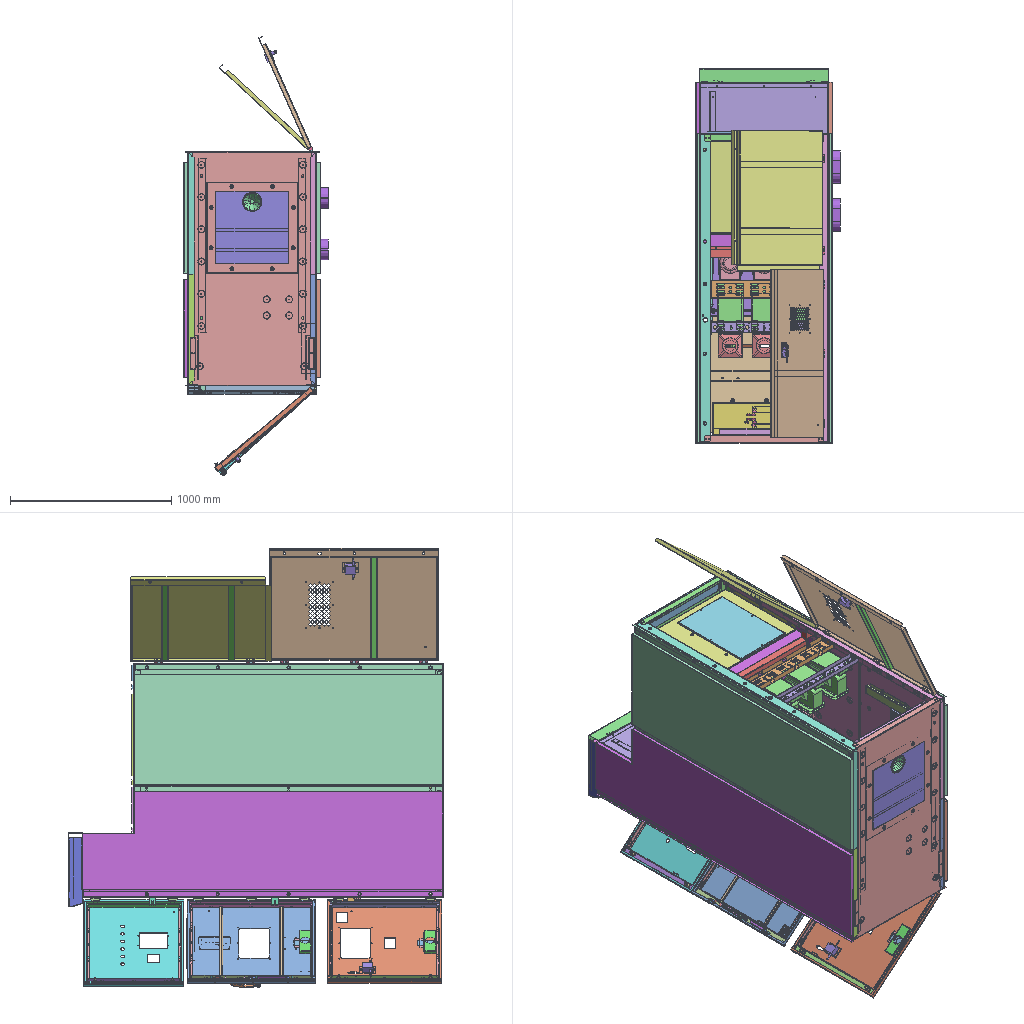Assembly | STEP file | 200 different items | 359 placed | box 898 x 2325 x 2724 mm
Parts list (item | name | quantity | parent item | size | volume):
1 | - | x1 | in Industrial electrical cabinet | 796 x 45 x 1450 mm | 2326374 mm3
2 | - | x1 | in Industrial electrical cabinet | 2240 x 691 x 80 mm | 4221901 mm3
3 | - | x1 | in Industrial electrical cabinet | 2240 x 691 x 80 mm | 4108988 mm3
4 | - | x1 | in Industrial electrical cabinet | 1920 x 759 x 80 mm | 3915251 mm3
5 | - | x1 | in Industrial electrical cabinet | 1920 x 759 x 80 mm | 2794848 mm3
6 | - | x1 | in Industrial electrical cabinet | 796 x 45 x 398 mm | 779012 mm3
7 | - | x1 | in Industrial electrical cabinet | 795 x 42 x 633 mm | 1100610 mm3
8 | - | x1 | in Industrial electrical cabinet | 796 x 45 x 1050 mm | 1045363 mm3
9 | - | x1 | in Industrial electrical cabinet | 795 x 88 x 393 mm | 764007 mm3
10 | - | x1 | in Industrial electrical cabinet | 660 x 140 x 682 mm | 1198837 mm3
11 | - | x1 | in Industrial electrical cabinet | 795 x 98 x 616 mm | 839757 mm3
12 | - | x1 | in Industrial electrical cabinet | 795 x 142 x 670 mm | 1317860 mm3
13 | - | x1 | in Industrial electrical cabinet | 46 x 30 x 440 mm | 87123 mm3
14 | Instrument cabinet room hinge | x4 | in Industrial electrical cabinet | 80 x 41 x 41 mm | 17041 mm3
15 | - | x1 | in Industrial electrical cabinet | 138 x 30 x 440 mm | 173584 mm3
16 | - | x1 | in Industrial electrical cabinet | 682 x 24 x 440 mm | 397013 mm3
17 | - | x1 | in Industrial electrical cabinet | 36 x 80 x 458 mm | 119357 mm3
18 | - | x2 | in Industrial electrical cabinet | 52 x 30 x 788 mm | 91760 mm3
19 | - | x2 | in Left guide rail assembly | 676 x 106.1 x 90 mm | 208424 mm3
20 | Left guide rail PN_0060 | x2 | in Left guide rail assembly | 686 x 80 x 19 mm | 166808 mm3
21 | - | x1 | in Right guide rail assembly | 676 x 106.1 x 90 mm | 208474 mm3
22 | - | x1 | in Right guide rail assembly | 587 x 51 x 15 mm | 62244 mm3
23 | Right guide rail PN_0062 | x1 | in Right guide rail assembly | 686 x 106 x 85 mm | 168135 mm3
24 | - | x2 | in Left support assembly, Right support assembly | 62 x 20 x 20 mm | 10868 mm3
25 | - | x4 | in Left support assembly, Right support assembly | 2.5 x 24 x 24 mm | 799.143 mm3
26 | - | x2 | in Left support assembly, Right support assembly | 25.5 x 25 x 25 mm | 5476 mm3
27 | - | x2 | in Left support assembly, Right support assembly | 24.52 x 27.353 x 1 mm | 170.96 mm3
28 | - | x2 | in Left support assembly, Right support assembly | 1 x 38 x 38 mm | 603.186 mm3
29 | - | x2 | in Left support assembly, Right support assembly | 13.58 x 15.928 x 1 mm | 67.493 mm3
30 | - | x2 | in Left support assembly, Right support assembly | 42 x 12 x 12 mm | 4112 mm3
31 | - | x2 | in Left support assembly, Right support assembly | 20 x 20 x 35 mm | 6555 mm3
32 | - | x4 | in Left support assembly, Right support assembly | 8.48 x 10.864 x 0.6 mm | 17.151 mm3
33 | - | x4 | in Left support assembly, Right support assembly | 1.6 x 16 x 16 mm | 233.031 mm3
34 | - | x2 | in Left support assembly, Right support assembly | 48 x 12 x 12 mm | 4791 mm3
35 | Shaft 4 PN_0052 | x2 | in Left support assembly, Right support assembly | 20 x 20 x 44 mm | 8364 mm3
36 | - | x4 | in Left support assembly, Right support assembly | 12 x 8 x 8 mm | 509.985 mm3
37 | - | x2 | in Industrial electrical cabinet | 378 x 18 x 80.5 mm | 66912 mm3
38 | - | x1 | in Industrial electrical cabinet | 378 x 18 x 80.5 mm | 66341 mm3
39 | - | x2 | in Industrial electrical cabinet | 690 x 18 x 35.5 mm | 51840 mm3
40 | - | x1 | in Industrial electrical cabinet | 789 x 25 x 775 mm | 895213 mm3
41 | - | x1 | in Industrial electrical cabinet | 739 x 43 x 710 mm | 942644 mm3
42 | - | x1 | in Industrial electrical cabinet | 740 x 26 x 428.5 mm | 502544 mm3
43 | Contact box type 150 | x6 | in Industrial electrical cabinet | 175.003 x 149 x 250 mm | 1890847 mm3
44 | - | x1 | in Industrial electrical cabinet | 700 x 15 x 151 mm | 151826 mm3
45 | - | x1 | in Industrial electrical cabinet | 700 x 15 x 562 mm | 498385 mm3
46 | - | x1 | in Industrial electrical cabinet | 700 x 15 x 279 mm | 263308 mm3
47 | 5.11.8.01.0013.1 DoorBeam | x1 | in Industrial electrical cabinet | 660 x 35 x 95 mm | 194127 mm3
48 | - | x1 | in Industrial electrical cabinet | 62 x 681 x 286 mm | 269371 mm3
49 | - | x2 | in Industrial electrical cabinet | 15 x 120 x 40.5 mm | 8986 mm3
50 | - | x13 | in Industrial electrical cabinet | 58.5 x 30 x 127 mm | 10567 mm3
51 | - | x1 | in Industrial electrical cabinet | 62 x 797 x 286 mm | 329890 mm3
52 | - | x1 | in Industrial electrical cabinet | 62 x 797 x 286 mm | 329072 mm3
53 | - | x1 | in Industrial electrical cabinet | 62 x 681 x 286 mm | 268904 mm3
54 | Bushing 110 x 180 | x3 | in Industrial electrical cabinet | 210 x 140 x 190 mm | 1953392 mm3
55 | A1 | x1 | in Industrial electrical cabinet | 155 x 100 x 289 mm | 478420 mm3
56 | B1 | x1 | in Industrial electrical cabinet | 305.057 x 100 x 289.003 mm | 480985 mm3
57 | C1 | x1 | in Industrial electrical cabinet | 305.395 x 100 x 28.803 mm | 306707 mm3
58 | C2 | x1 | in Industrial electrical cabinet | 100 x 800 x 10 mm | 800000 mm3
59 | A2 | x1 | in Industrial electrical cabinet | 100 x 800 x 10 mm | 800000 mm3
60 | B2 | x1 | in Industrial electrical cabinet | 100 x 800 x 10 mm | 800000 mm3
61 | Rear lower door (upper/lower interlock) | x1 | in Rear lower door (upper/lower interlock) assembly | 748.5 x 1045 x 28 mm | 1316932 mm3
62 | DSN-BMZ indoor electromagnetic lock | x3 | in Rear lower door (upper/lower interlock) assembly, Industrial electrical cabinet | 137 x 126 x 78.5 mm | 180321 mm3
63 | Rear door reinforcing rib | x3 | in Rear lower door (upper/lower interlock) assembly, Rear upper door (upper/lower interlock) assembly | 40 x 691 x 23.5 mm | 85064 mm3
64 | 5.11.8.01.1033.1 Bracket(Right) | x1 | in Industrial electrical cabinet | 42 x 45 x 1080 mm | 235963 mm3
65 | 5.11.8.01.1032.1 Bracket(Left) | x1 | in Industrial electrical cabinet | 42 x 45 x 1080 mm | 235914 mm3
66 | - | x2 | in Industrial electrical cabinet | 40 x 50 x 640 mm | 121890 mm3
67 | - | x3 | in Industrial electrical cabinet | 42 x 40 x 640 mm | 101667 mm3
68 | Earthing switch reinforcing rib | x1 | in Industrial electrical cabinet | 785 x 20 x 65 mm | 208517 mm3
69 | 8XS043017.1~5 | x1 | - | 315 x 116 x 140 mm | 129914 mm3
70 | 8XS161060 | x1 | in 5XS174017 | 72 x 65 x 65 mm | 16979 mm3
71 | 8XS234010 | x1 | in 5XS174017 | 8 x 110.249 x 97 mm | 8595 mm3
72 | 8XS200020 | x1 | - | 8 x 8 x 85 mm | 4231 mm3
73 | 8XS224021_8GD.211.061 | x1 | - | 16.1 x 26.2 x 26.2 mm | 7800 mm3
74 | 8XS900010 | x1 | - | 10 x 14 x 32 mm | 1489 mm3
75 | spring lock washers--normal type gb_GB_FASTENER_WASHER_SW 5 | x1 | - | 8 x 8 x 1.3 mm | 34.298 mm3
76 | hex nuts, style 1-grades ab gb_GB_FASTENER_NUT_SNAB1 M5-S | x1 | - | 9.238 x 8 x 4.7 mm | 181.423 mm3
77 | plain washers--product grade c gb_GB_FASTENER_WASHER_SMWC 5 | x1 | - | 10 x 10 x 1 mm | 54.782 mm3
78 | JZ-58 secondary plug socket | x1 | - | 225 x 81 x 134.749 mm | 1282541 mm3
79 | - | x1 | in Industrial electrical cabinet | 42.8 x 780 x 125 mm | 154467 mm3
80 | Small busbar cover (flat top flange) | x1 | in Industrial electrical cabinet | 798 x 59 x 377 mm | 518069 mm3
81 | - | x2 | in Industrial electrical cabinet | 75 x 40 x 2 mm | 5167 mm3
82 | Earthing switch operating hole label | x1 | in Industrial electrical cabinet | 119 x 38 x 2 mm | 6366 mm3
83 | - | x1 | in Industrial electrical cabinet | 565 x 12 x 565 mm | 496282 mm3
84 | - | x1 | in Industrial electrical cabinet | 697 x 59 x 30 mm | 98797 mm3
85 | - | x1 | in Industrial electrical cabinet | 682 x 24 x 440 mm | 453333 mm3
86 | Large bent plate rear cover | x1 | in Industrial electrical cabinet | 555 x 10 x 390 mm | 277878 mm3
87 | Zero-sequence current transformer mounting plate | x1 | in Industrial electrical cabinet | 50 x 200 x 640 mm | 327853 mm3
88 | Cable clamp | x1 | in Industrial electrical cabinet | 60 x 75 x 115 mm | 247927 mm3
89 | Tower-type sealing ring | x1 | in Industrial electrical cabinet | 120 x 60.067 x 120 mm | 130972 mm3
90 | - | x1 | in Industrial electrical cabinet | 731.5 x 98.5 x 68.5 mm | 147735 mm3
91 | Heater | x1 | in Industrial electrical cabinet | 180 x 20 x 100 mm | 172535 mm3
92 | 8XS123012 | x3 | in PN_0063 (for VS1) | 52 x 48 x 30 mm | 9095 mm3
93 | 8XS123013 | x3 | in PN_0063 (for VS1) | 52 x 48 x 30 mm | 9095 mm3
94 | 8XS320011-1~2_8XS320011.2 | x1 | in PN_0063 (for VS1) | 682 x 145 x 38.3 mm | 150091 mm3
95 | 8XS320010-1~2_8XS320010.2 | x1 | in PN_0063 (for VS1) | 682 x 145 x 38 mm | 186768 mm3
96 | 8XS234011 | x2 | in PN_0063 (for VS1) | 10 x 750 x 10 mm | 58101 mm3
97 | 8XS210011 | x2 | in PN_0063 (for VS1) | 10 x 20 x 20 mm | 2271 mm3
98 | 8XS100010 | x1 | in 5XS100010 | 95 x 55 x 50 mm | 28104 mm3
99 | 8XS200017 | x2 | in 5XS100010, 5XS100011 | 62 x 20 x 20 mm | 10868 mm3
100 | 8XS174012 | x1 | in 5XS174012 | 13 x 81 x 207 mm | 21845 mm3
101 | 8XS211050 | x2 | in 5XS174012, 5XS174011 | 25.5 x 25 x 25 mm | 5476 mm3
102 | 8XS200013-1 | x2 | in 5XS174012, 5XS174011 | 42 x 12 x 12 mm | 4112 mm3
103 | 8XS200016 | x4 | in 5XS174012, 5XS174013, 5XS174011, 5XS174014 | 12 x 8 x 8 mm | 509.985 mm3
104 | 8XS174010 | x1 | in 5XS174013 | 13 x 81 x 207 mm | 22375 mm3
105 | 8XS210010 | x2 | in 5XS174013, 5XS174014 | 26 x 18 x 18 mm | 3420 mm3
106 | 8XS200013-2 | x2 | in 5XS174013, 5XS174014 | 48 x 12 x 12 mm | 4791 mm3
107 | TES_Plain washer GB 97.1 12 | x4 | in 5XS235010, 5XS235011 | 2.5 x 24 x 24 mm | 799.143 mm3
108 | 8XS156012 | x2 | in 5XS235010, 5XS235011 | 1 x 38 x 38 mm | 603.186 mm3
109 | TES_Plain washer GB 97.1 8 | x4 | in 5XS235010, 5XS235011 | 1.6 x 16 x 16 mm | 233.031 mm3
110 | GB 894.1-86 7 | x4 | in 5XS235010, 5XS235011 | 8.48 x 10.864 x 0.6 mm | 17.151 mm3
111 | GB 894.1-86 12 | x2 | in 5XS235010, 5XS235011 | 13.58 x 15.928 x 1 mm | 67.493 mm3
112 | Circlip GB 894.1-86 22 | x2 | in 5XS235010, 5XS235011 | 24.52 x 27.353 x 1 mm | 170.96 mm3
113 | 8XS210012-4 | x2 | in 5XS235010, 5XS235011 | 20 x 20 x 44 mm | 8364 mm3
114 | 8XS210012-3 | x2 | in 5XS235010, 5XS235011 | 20 x 20 x 35 mm | 6555 mm3
115 | 8XS100011 | x1 | in 5XS100011 | 95 x 55 x 50 mm | 28104 mm3
116 | 8XS174013 | x1 | in 5XS174011 | 13 x 81 x 207 mm | 21986 mm3
117 | 8XS174011 | x1 | in 5XS174014 | 13 x 81 x 207 mm | 22375 mm3
118 | 8XS123010 | x1 | in PN_0063 (for VS1) | 115 x 112 x 34 mm | 22620 mm3
119 | 8XS123011 | x1 | in PN_0063 (for VS1) | 115 x 112 x 34 mm | 22620 mm3
120 | 8XS174017-2B | x2 | in 5XS174015-2 | 20 x 510 x 16 mm | 32373 mm3
121 | 8XS200018 | x4 | in 5XS174015-2, 5XS174016-2 | 8 x 8 x 11 mm | 446.551 mm3
122 | 8XS174016-2 | x2 | in 5XS174016-2 | 16 x 127 x 4 mm | 7662 mm3
123 | - | x1 | in Left guide rail assembly | 587 x 51 x 15 mm | 63282 mm3
124 | 8XS161064 | x1 | in 5XS260010 | 686 x 106 x 85 mm | 168135 mm3
125 | 8XS161066 | x1 | in 5XS260010 | 676 x 106.1 x 90 mm | 208474 mm3
126 | 8XS161062 | x1 | in 5XS260010 | 587 x 51 x 15 mm | 62244 mm3
127 | Electromagnetic lock bracket A | x1 | in Industrial electrical cabinet | 15 x 56 x 50 mm | 6308 mm3
128 | Bottom plate secondary wiring hole cover | x1 | in Industrial electrical cabinet | 90 x 2 x 310 mm | 55646 mm3
129 | Small busbar cover | x1 | in Industrial electrical cabinet | 798 x 87 x 420 mm | 602724 mm3
130 | Top flange baffle | x1 | in Industrial electrical cabinet | 423.333 x 35 x 81 mm | 59476 mm3
131 | Top flange (flat door) AA | x1 | in Industrial electrical cabinet | 77.333 x 86 x 798 mm | 299938 mm3
132 | 15 | x1 | - | 8 x 175 x 150 mm | 26708 mm3
133 | 18 | x1 | - | 12 x 62.5 x 12 mm | 2879 mm3
134 | 13 | x1 | - | 25 x 128 x 30 mm | 12857 mm3
135 | 8xs161054 | x1 | - | 60 x 30 x 20 mm | 6156 mm3
136 | 8xs043021 | x1 | - | 55 x 34 x 24 mm | 17004 mm3
137 | 8xs200012 | x1 | - | 6 x 8 x 80 mm | 3378 mm3
138 | spring pin slotted light duty1 gb | x1 | - | 20 x 3 x 2.985 mm | 48.044 mm3
139 | 8xs282020 | x1 | - | 11 x 11 x 33.6 mm | 193.342 mm3
140 | - | x1 | - | 33 x 185 x 210 mm | 62468 mm3
141 | - | x1 | - | 220 x 25 x 35 mm | 17944 mm3
142 | 2  spring | x1 | - | 17 x 17 x 62.598 mm | 2374 mm3
143 | - | x2 | - | 22 x 125 x 40 mm | 9938 mm3
144 | - | x1 | - | 10 x 32 x 45.5 mm | 7902 mm3
145 | - | x1 | - | 11.547 x 10 x 55 mm | 1784 mm3
146 | Top flange baffle (inner bend) | x1 | in Industrial electrical cabinet | 422.833 x 35 x 83 mm | 73791 mm3
147 | - | x1 | in Industrial electrical cabinet | 713.5 x 64.5 x 74.5 mm | 87062 mm3
148 | Channel plate (instrument transformer) | x1 | in Industrial electrical cabinet | 659.8 x 110 x 35 mm | 157796 mm3
149 | Channel plate 2 | x1 | in Industrial electrical cabinet | 659.8 x 70 x 32 mm | 159810 mm3
150 | Current transformer LZZJ9-10Q | x3 | in Industrial electrical cabinet | 295 x 230 x 160 mm | 6235515 mm3
151 | Hinge side | x5 | in Hinge assembly 1 | 19 x 29 x 51 mm | 16162 mm3
152 | Hinge middle | x5 | in Hinge assembly 1 | 18 x 51 x 16 mm | 8751 mm3
153 | Rear upper door (upper/lower interlock) | x1 | in Rear upper door (upper/lower interlock) assembly | 748.5 x 873.5 x 28 mm | 1158666 mm3
154 | - | x1 | in Industrial electrical cabinet | 697 x 2240 x 25 mm | 2428622 mm3
155 | Cover plate 2 | x2 | in Industrial electrical cabinet | 790 x 1920 x 25 mm | 2483939 mm3
156 | Cover plate 3 | x1 | in Industrial electrical cabinet | 697 x 2240 x 25 mm | 2429916 mm3
157 | Top flange baffle 2 | x1 | in Industrial electrical cabinet | 422.83 x 83 x 35 mm | 73586 mm3
158 | Hinge base | x7 | in Front door hinge assembly | 51 x 34 x 60 mm | 23679 mm3
159 | Hinge movable plate | x7 | in Front door hinge assembly | 34 x 28.999 x 60 mm | 17414 mm3
160 | - | x1 | - | 775 x 32 x 620 mm | 1109969 mm3
161 | Cylinder lock | x4 | - | 50 x 30 x 30 mm | 11941 mm3
162 | Instrument door gasket strip vertical (lock hole) modified | x1 | - | 44.5 x 615 x 28.5 mm | 95558 mm3
163 | Instrument door gasket strip vertical (hinge) modified | x1 | - | 44.5 x 615 x 28.5 mm | 98883 mm3
164 | Gasket strip horizontal (flat door) modified | x6 | - | 28.5 x 684 x 12 mm | 48634 mm3
165 | - | x1 | - | 775 x 32 x 796 mm | 1362848 mm3
166 | Pin | x3 | in Assembly (middle door pull rod lock) | 10 x 10 x 58 mm | 3562 mm3
167 | Pull rod connecting plate | x1 | in Assembly (middle door pull rod lock) | 120 x 20 x 32 mm | 7229 mm3
168 | - | x1 | in Assembly (middle door pull rod lock) | 39.772 x 190 x 20.1 mm | 27752 mm3
169 | - | x1 | in Assembly (middle door pull rod lock) | 193.54 x 37.8 x 32 mm | 42098 mm3
170 | Nut MS887-3-4 | x1 | in Assembly (middle door pull rod lock) | 27 x 4 x 31.177 mm | 789.045 mm3
171 | - | x1 | in Assembly (middle door pull rod lock) | 22 x 33 x 38.56 mm | 10259 mm3
172 | - | x2 | in Assembly (middle door pull rod lock) | 6 x 28.229 x 44 mm | 2102 mm3
173 | - | x1 | in Assembly (middle door pull rod lock) | 6 x 6 x 11.5 mm | 323.208 mm3
174 | - | x2 | in Assembly (middle door pull rod lock) | 6 x 6 x 20 mm | 563.539 mm3
175 | Lower pull rod (lower door)_6 | x1 | in Assembly (middle door pull rod lock) | 300 x 18 x 29.5 mm | 15254 mm3
176 | Lower pull rod (lower door)_4 | x1 | in Assembly (middle door pull rod lock) | 21.5 x 18 x 23 mm | 1390 mm3
177 | Upper pull rod (lower door) | x1 | in Assembly (middle door pull rod lock) | 98 x 18 x 28 mm | 4727 mm3
178 | - | x3 | in Assembly (middle door pull rod lock) | 25 x 23.5 x 12 mm | 5803 mm3
179 | Middle door gasket strip vertical (door lock) modified | x1 | - | 44.5 x 791 x 28.5 mm | 124119 mm3
180 | Middle door gasket strip vertical (hinge) modified | x1 | - | 44.5 x 791 x 28.5 mm | 125821 mm3
181 | 8ZY.143.1010 | x3 | - | 20 x 45 x 10 mm | 4499 mm3
182 | Door reinforcing rib (flat door) modified U | x2 | - | 20 x 684 x 12 mm | 51617 mm3
183 | Insert/withdraw label (with lock) | x2 | - | 102 x 72 x 3.5 mm | 19316 mm3
184 | Slide plate seat | x2 | - | 200 x 42 x 75 mm | 42985 mm3
185 | Slide plate bracket | x2 | - | 160 x 30 x 20 mm | 8510 mm3
186 | Slide plate | x2 | - | 48 x 20 x 97 mm | 9605 mm3
187 | Warning label | x1 | - | - | 14089 mm3
188 | - | x1 | - | 463 x 15 x 50 mm | 57863 mm3
189 | Mimic panel | x1 | - | 125 x 195 x 2 mm | 47954 mm3
190 | - | x1 | - | 775 x 32 x 710 mm | 1181727 mm3
191 | Lower door gasket strip vertical (hinge) modified | x1 | - | 44.5 x 705 x 28.5 mm | 113772 mm3
192 | Lower door gasket strip vertical (door lock) modified | x1 | - | 44.5 x 705 x 28.5 mm | 109938 mm3
193 | LXZK120 | x1 | in Industrial electrical cabinet | 280 x 252 x 144 mm | 2421478 mm3
194 | High voltage insulator | x3 | in Industrial electrical cabinet | 80 x 140 x 80 mm | 533593 mm3
195 | Transformer bracket | x2 | in Industrial electrical cabinet | 50 x 640 x 20 mm | 94677 mm3
196 | JDZJ(X)10-10(R)(L) series voltage transformer(1).step | x2 | in Industrial electrical cabinet | 326.1 x 237.96 x 160 mm | 7233561 mm3
197 | Through tube 95 | x3 | in Industrial electrical cabinet | 150 x 264.782 x 150 mm | 1178691 mm3
198 | Surge arrester | x3 | in Surge arrester assembly | 242 x 92.835 x 92.835 mm | 456691 mm3
199 | Surge arrester washer | x12 | in Surge arrester assembly | 21 x 21 x 2 mm | 502.655 mm3
200 | Surge arrester nut | x6 | in Surge arrester assembly | 20.659 x 19.032 x 8 mm | 1616 mm3
Placements (level | parent | child | x y z in mm | rotation matrix by rows), first 329 of 403 lines:
1 | Industrial electrical cabinet | subassembly 2 | -5197.537 106.592 -4409.824 | 1 0 0 0 1 0 0 0 1
1 | Industrial electrical cabinet | subassembly 3 | -4401.537 104.592 -5855.824 | 0 0 1 1 0 0 0 1 -0
1 | Industrial electrical cabinet | subassembly 4 | -5199.537 104.592 -5855.824 | 0 0 1 1 0 0 0 1 0
1 | Industrial electrical cabinet | subassembly 5 | -4403.537 104.592 -4409.824 | 0 0 -1 1 0 0 0 -1 0
1 | Industrial electrical cabinet | subassembly 6 | -5201.537 104.592 -4409.824 | 0 0 -1 1 0 0 0 -1 -0
1 | Industrial electrical cabinet | subassembly 7 | -5199.537 2338.592 -5855.824 | 1 0 0 0 -1 0 0 0 -1
1 | Industrial electrical cabinet | subassembly 8 | -5199.037 1702.592 -5457.824 | 1 0 0 0 0 -1 0 1 0
1 | Industrial electrical cabinet | subassembly 9 | -4403.537 2018.592 -4409.824 | -1 0 0 0 -1 0 0 0 1
1 | Industrial electrical cabinet | subassembly 10 | -5199.037 1702.592 -5461.824 | 1 0 0 0 1 0 0 0 1
1 | Industrial electrical cabinet | subassembly 11 | -5131.637 931.592 -5175.824 | 1 0 0 0 1 0 0 0 1
1 | Industrial electrical cabinet | subassembly 12 | -4406.037 1402.592 -4538.824 | -1 0 0 0 0 -1 0 -1 0
1 | Industrial electrical cabinet | subassembly 13 | -5197.037 1300.592 -4536.824 | 1 0 0 0 1 0 0 0 1
1 | Industrial electrical cabinet | subassembly 14 | -4407.537 1840.592 -5681.824 | -1 0 0 0 0 -1 0 -1 -0
1 | Industrial electrical cabinet | Instrument cabinet room hinge | -4455.037 1850.592 -5671.824 | 0 0 1 -1 0 0 0 -1 -0
1 | Industrial electrical cabinet | Instrument cabinet room hinge | -4455.037 2190.592 -5671.824 | 0 0 1 -1 0 0 0 -1 -0
1 | Industrial electrical cabinet | subassembly 15 | -4443.037 2280.592 -5670.324 | 0 1 0 0 0 1 1 0 0
1 | Industrial electrical cabinet | Instrument cabinet room hinge | -4455.037 1850.592 -5530.824 | 0 1 0 -1 0 0 0 0 1
1 | Industrial electrical cabinet | Instrument cabinet room hinge | -4455.037 2190.592 -5530.824 | 0 1 0 -1 0 0 0 0 1
1 | Industrial electrical cabinet | subassembly 16 | -5138.537 1840.592 -5519.324 | 1 0 0 0 0 -1 0 1 -0
1 | Industrial electrical cabinet | subassembly 17 | -5102.537 2286.592 -5509.824 | -1 0 0 0 0 1 0 1 -0
1 | Industrial electrical cabinet | subassembly 18 | -4407.537 1750.886 -5732.747 | 0 0 1 0.342 -0.9397 0 0.9397 0.342 -0
1 | Industrial electrical cabinet | subassembly 18 | -4407.537 1750.886 -5607.747 | 0 0 1 0.342 -0.9397 0 0.9397 0.342 -0
1 | Industrial electrical cabinet | Left guide rail assembly | -4410.227 1115.203 -6154.732 | 0 0 -1 0 1 0 1 0 -0
2 | Left guide rail assembly | subassembly 19 | 311.908 -202.611 59.31 | 1 0 0 0 1 0 0 0 1
2 | Left guide rail assembly | Left guide rail PN_0060 | 301.908 -180.611 61.31 | 1 0 0 0 1 0 0 0 1
1 | Industrial electrical cabinet | Right guide rail assembly | -5131.537 912.592 -5842.824 | 0 0 -1 0 1 0 1 0 -0
2 | Right guide rail assembly | subassembly 20 | -0.0 -0.0 -0.0 | 1 0 0 0 1 0 0 0 1
2 | Right guide rail assembly | subassembly 21 | 607.0 62.0 -3.0 | -1 0 0 0 1 0 0 0 -1
2 | Right guide rail assembly | Right guide rail PN_0062 | 666.0 22.0 -0.0 | -1 0 0 0 1 0 0 0 -1
1 | Industrial electrical cabinet | Left support assembly | -4407.537 1033.092 -5432.824 | 0 0 -1 0 1 0 1 0 0
2 | Left support assembly | subassembly 22 | 45.0 19.5 -0.0 | 0 0.383 0.9237 0 -0.9237 0.383 1 0 -0
2 | Left support assembly | subassembly 23 | 45.0 19.5 23.0 | 0 0 -1 0 1 0 1 0 -0
2 | Left support assembly | subassembly 23 | 45.0 19.5 54.0 | 0 0 -1 0 1 0 1 0 -0
2 | Left support assembly | subassembly 24 | 45.0 19.5 54.0 | 0 0 1 0 1 0 -1 0 0
2 | Left support assembly | subassembly 25 | 45.0 20.17 31.5 | 1 0 0 0 1 0 0 0 1
2 | Left support assembly | subassembly 26 | 45.0 19.5 32.5 | 0 0 -1 0 1 0 1 0 -0
2 | Left support assembly | subassembly 27 | 45.0 19.93 57.0 | 1 0 0 0 1 0 0 0 1
2 | Left support assembly | subassembly 28 | 45.0 64.5 41.0 | 0 0 -1 0 1 0 1 0 -0
2 | Left support assembly | subassembly 29 | 45.0 64.5 47.0 | 1 0 0 0 1 0 0 0 1
2 | Left support assembly | subassembly 30 | 45.0 64.5 80.5 | 1 0 0 0 1 0 0 0 1
2 | Left support assembly | subassembly 30 | 45.0 -25.5 81.0 | 1 0 0 0 1 0 0 0 1
2 | Left support assembly | subassembly 31 | 45.0 64.5 78.9 | 0 0 -1 0 1 0 1 0 -0
2 | Left support assembly | subassembly 31 | 45.0 -25.5 81.0 | 0 0 1 0 1 0 -1 0 0
2 | Left support assembly | subassembly 32 | 45.0 -25.5 35.5 | 0 0 -1 0 1 0 1 0 -0
2 | Left support assembly | Shaft 4 PN_0052 | 45.0 -25.5 39.0 | 1 0 0 0 1 0 0 0 1
2 | Left support assembly | subassembly 33 | 226.0 74.5 41.0 | 0 0 -1 0 1 0 1 0 -0
2 | Left support assembly | subassembly 33 | 226.0 -35.5 38.5 | 0 0 1 0 1 0 -1 0 0
1 | Industrial electrical cabinet | Right support assembly | -5246.721 1035.998 -5444.702 | 0 0 -1 0 1 0 1 0 -0
2 | Right support assembly | subassembly 23 | 56.878 16.594 -76.683 | 0 0 -1 0 1 0 1 0 0
2 | Right support assembly | subassembly 23 | 56.878 16.594 -105.683 | 0 0 1 0 1 0 -1 0 -0
2 | Right support assembly | subassembly 27 | 56.713 16.991 -108.183 | -0.9237 -0.383 0 -0.383 0.9237 0 0 0 -1
2 | Right support assembly | subassembly 28 | 56.878 61.594 -92.683 | 0 -0.383 0.9237 0 0.9237 0.383 -1 0 0
2 | Right support assembly | subassembly 29 | 56.878 61.594 -98.683 | -0.9237 -0.383 0 -0.383 0.9237 0 0 0 -1
2 | Right support assembly | subassembly 30 | 56.878 61.594 -132.184 | -0.9237 -0.383 0 -0.383 0.9237 0 0 0 -1
2 | Right support assembly | subassembly 30 | 56.878 -28.406 -132.184 | -0.9237 -0.383 0 -0.383 0.9237 0 0 0 -1
2 | Right support assembly | subassembly 31 | 56.878 61.594 -130.583 | 0 -0.383 0.9237 0 0.9237 0.383 -1 0 0
2 | Right support assembly | subassembly 31 | 56.878 -28.406 -132.184 | 0 -0.383 -0.9237 0 0.9237 -0.383 1 0 -0
2 | Right support assembly | subassembly 32 | 56.878 -28.406 -86.683 | 0 -0.383 0.9237 0 0.9237 0.383 -1 0 0
2 | Right support assembly | Shaft 4 PN_0052 | 56.878 -28.406 -90.183 | -0.9237 -0.383 0 -0.383 0.9237 0 0 0 -1
2 | Right support assembly | subassembly 22 | 56.878 16.594 -51.184 | 0 0.383 -0.9237 0 -0.9237 -0.383 -1 0 0
2 | Right support assembly | subassembly 24 | 56.878 16.594 -105.683 | 0 0 -1 0 1 0 1 0 0
2 | Right support assembly | subassembly 25 | 56.878 17.264 -84.183 | 1 0 0 0 1 0 0 0 1
2 | Right support assembly | subassembly 26 | 56.878 16.594 -84.183 | 0 0 1 0 1 0 -1 0 -0
2 | Right support assembly | subassembly 33 | 237.878 71.594 -92.683 | 0 0 1 0 1 0 -1 0 -0
2 | Right support assembly | subassembly 33 | 237.878 -38.406 -89.683 | 0 0 -1 0 1 0 1 0 0
1 | Industrial electrical cabinet | subassembly 34 | -4425.537 832.592 -5169.824 | 0 -1 0 0 0 1 -1 0 0
1 | Industrial electrical cabinet | subassembly 35 | -5115.934 883.549 -6392.689 | 0 1 0 0 0 1 1 0 -0
1 | Industrial electrical cabinet | subassembly 36 | -5177.537 832.092 -5159.824 | 0 1 0 0 0 1 1 0 0
1 | Industrial electrical cabinet | subassembly 36 | -4425.537 831.748 -4474.008 | 0 -1 0 0 0 1 -1 0 0
1 | Industrial electrical cabinet | subassembly 37 | -4408.537 117.592 -5170.324 | -1 0 0 0 0 -1 0 -1 -0
1 | Industrial electrical cabinet | subassembly 38 | -4434.037 892.592 -5170.824 | -1 0 0 0 0 -1 0 -1 0
1 | Industrial electrical cabinet | subassembly 39 | -4431.537 1603.592 -5170.324 | -1 0 0 0 0 -1 0 -1 0
1 | Industrial electrical cabinet | Contact box type 150 | -5011.584 1492.594 -5168.824 | 0 1 0 -1 0 0 0 0 1
1 | Industrial electrical cabinet | Contact box type 150 | -4801.584 1492.594 -5168.824 | 0 1 0 -1 0 0 0 0 1
1 | Industrial electrical cabinet | Contact box type 150 | -5011.59 1217.589 -5168.824 | 0 -1 0 1 0 0 0 0 1
1 | Industrial electrical cabinet | Contact box type 150 | -4801.59 1217.589 -5168.824 | 0 -1 0 1 0 0 0 0 1
1 | Industrial electrical cabinet | Contact box type 150 | -4591.59 1217.589 -5168.824 | 0 -1 0 1 0 0 0 0 1
1 | Industrial electrical cabinet | Contact box type 150 | -4591.584 1492.594 -5168.824 | 0 1 0 -1 0 0 0 0 1
1 | Industrial electrical cabinet | subassembly 40 | -4353.537 2021.792 -4788.824 | -1 0 0 0 1 0 0 0 -1
1 | Industrial electrical cabinet | subassembly 41 | -4353.537 2021.792 -4969.824 | -1 0 0 0 1 0 0 0 -1
1 | Industrial electrical cabinet | subassembly 42 | -4352.989 2021.792 -5547.996 | -1 0 0 0 1 0 0 0 -1
1 | Industrial electrical cabinet | 5.11.8.01.0013.1 DoorBeam | -5131.437 1663.092 -5855.824 | 1 0 0 0 0 -1 0 1 0
1 | Industrial electrical cabinet | subassembly 43 | -4470.437 898.136 -4930.925 | 1 0 0 0 1 0 0 0 1
1 | Industrial electrical cabinet | subassembly 44 | -4407.537 2028.991 -5280.868 | 1 0 0 0 0 1 0 -1 -0
1 | Industrial electrical cabinet | subassembly 45 | -4466.037 1284.547 -4893.925 | -1 0 0 0 -1 0 0 0 1
1 | Industrial electrical cabinet | subassembly 45 | -4466.037 1634.547 -4893.925 | -1 0 0 0 -1 0 0 0 1
1 | Industrial electrical cabinet | subassembly 45 | -5137.037 1284.547 -6576.723 | 1 0 0 0 -1 0 0 0 -1
1 | Industrial electrical cabinet | subassembly 45 | -4466.037 1114.193 -5625.868 | -1 0 0 0 0 -1 0 -1 -0
1 | Industrial electrical cabinet | subassembly 45 | -4466.037 1309.193 -5625.868 | -1 0 0 0 0 -1 0 -1 0
1 | Industrial electrical cabinet | subassembly 46 | -4470.437 -4.364 -4930.925 | 1 0 0 0 1 0 0 0 1
1 | Industrial electrical cabinet | subassembly 45 | -4466.037 414.547 -4893.925 | -1 0 0 0 -1 0 0 0 1
1 | Industrial electrical cabinet | subassembly 45 | -4466.037 694.547 -4893.925 | -1 0 0 0 -1 0 0 0 1
1 | Industrial electrical cabinet | subassembly 47 | -5131.437 -4.364 -4930.925 | 1 0 0 0 1 0 0 0 1
1 | Industrial electrical cabinet | subassembly 45 | -5137.037 414.547 -6576.723 | 1 0 0 0 -1 0 0 0 -1
1 | Industrial electrical cabinet | subassembly 45 | -5137.037 694.547 -6576.723 | 1 0 0 0 -1 0 0 0 -1
1 | Industrial electrical cabinet | subassembly 44 | -5195.537 2028.991 -5634.78 | -1 0 0 0 0 1 0 1 0
1 | Industrial electrical cabinet | subassembly 48 | -5131.437 898.136 -4930.925 | 1 0 0 0 1 0 0 0 1
1 | Industrial electrical cabinet | subassembly 45 | -5137.037 1634.547 -6576.723 | 1 0 0 0 -1 0 0 0 -1
1 | Industrial electrical cabinet | Bushing 110 x 180 | -4428.537 1879.593 -5064.133 | 0 0 1 -1 0 0 0 -1 0
1 | Industrial electrical cabinet | Bushing 110 x 180 | -4428.537 1879.593 -4744.133 | 0 0 1 -1 0 0 0 -1 -0
1 | Industrial electrical cabinet | Bushing 110 x 180 | -4428.537 1579.593 -4744.133 | 0 0 1 -1 0 0 0 -1 0
1 | Industrial electrical cabinet | A1 | -4541.584 1562.594 -4978.824 | 0 -1 0 1 0 0 0 0 1
1 | Industrial electrical cabinet | B1 | -4751.584 1562.594 -4978.824 | 0 -1 0 1 0 0 0 0 1
1 | Industrial electrical cabinet | C1 | -4961.584 1562.594 -4978.824 | 0 -1 0 1 0 0 0 0 1
1 | Industrial electrical cabinet | C2 | -5201.537 1867.592 -5008.824 | 0 1 0 -1 0 0 0 0 1
1 | Industrial electrical cabinet | A2 | -5201.537 1567.592 -4688.824 | 0 1 0 -1 0 0 0 0 1
1 | Industrial electrical cabinet | B2 | -5201.537 1867.592 -4688.824 | 0 1 0 -1 0 0 0 0 1
1 | Industrial electrical cabinet | Rear lower door (upper/lower interlock) assembly | -721.878 -862.327 2034.777 | 0.9145 0 -0.4046 0 1 0 0.4046 0 0.9145
2 | Rear lower door (upper/lower interlock) assembly | Rear lower door (upper/lower interlock) | -5989.032 996.519 -3660.045 | 0 0 -1 0 1 0 1 0 0
2 | Rear lower door (upper/lower interlock) assembly | DSN-BMZ indoor electromagnetic lock | -6025.532 1509.519 -3719.545 | 0 0 1 0 1 0 -1 0 -0
2 | Rear lower door (upper/lower interlock) assembly | Rear door reinforcing rib | -6011.032 1376.519 -3662.545 | 0 0 1 -1 0 0 0 -1 -0
1 | Industrial electrical cabinet | 5.11.8.01.1033.1 Bracket(Right) | -5088.537 110.592 -4447.824 | 0 -1 0 1 0 0 0 0 1
1 | Industrial electrical cabinet | 5.11.8.01.1032.1 Bracket(Left) | -4574.302 65.387 -3829.974 | 0 1 0 -1 0 0 0 0 1
1 | Industrial electrical cabinet | subassembly 49 | -4481.537 202.592 -5121.361 | 0 0 1 0 -1 0 1 0 0
1 | Industrial electrical cabinet | subassembly 50 | -4481.537 154.592 -4901.628 | 0 0 1 0 -1 0 1 0 0
1 | Industrial electrical cabinet | subassembly 50 | -4481.537 154.592 -5026.628 | 0 0 1 0 -1 0 1 0 0
1 | Industrial electrical cabinet | Earthing switch reinforcing rib | -5194.037 552.592 -5172.824 | 1 0 0 0 0 1 0 -1 0
1 | Industrial electrical cabinet | subassembly 51 | -4963.623 1627.909 -5608.076 | -1 0 0 0 1 0 0 0 -1
2 | subassembly 51 | 8XS043017.1~5 | -191.086 -43.318 17.748 | 1 0 0 0 1 0 0 0 1
2 | subassembly 51 | 5XS174017 | 90.475 -20.442 36.677 | -1 0 0 0 0.0344 -0.9994 0 -0.9994 -0.0344
3 | 5XS174017 | 8XS161060 | -29.44 32.426 -39.738 | 1 0 0 0 1 0 0 0 1
3 | 5XS174017 | 8XS234010 | 14.56 -29.574 -14.738 | 0 1 0 0 0 -1 -1 0 -0
2 | subassembly 51 | 8XS200020 | 126.414 -6.318 54.748 | 0 0 -1 0.7786 -0.6275 0 -0.6275 -0.7786 -0
2 | subassembly 51 | 8XS224021_8GD.211.061 | 110.914 -37.095 18.668 | 1 0 0 0 0.721 0.693 0 -0.693 0.721
2 | subassembly 51 | 8XS900010 | 100.814 -37.095 18.668 | 0 0 -1 0.139 0.9903 0 0.9903 -0.139 -0
2 | subassembly 51 | spring lock washers--normal type gb_GB_FASTENER_WASHER_SW 5 | 122.214 -37.095 18.668 | 0 0 1 0 1 0 -1 0 0
2 | subassembly 51 | hex nuts, style 1-grades ab gb_GB_FASTENER_NUT_SNAB1 M5-S | 126.914 -37.095 18.668 | 0 0 1 0 1 0 -1 0 0
2 | subassembly 51 | plain washers--product grade c gb_GB_FASTENER_WASHER_SMWC 5 | 119.914 -37.095 18.668 | 0 0 -1 -0.1555 0.9878 0 0.9878 0.1555 -0
2 | subassembly 51 | JZ-58 secondary plug socket | -68.086 -2.318 17.748 | 1 0 0 0 1 0 0 0 1
1 | Industrial electrical cabinet | subassembly 52 | -4294.582 2461.991 -5495.024 | 0 -1 0 0 0 1 -1 0 0
1 | Industrial electrical cabinet | Small busbar cover (flat top flange) | -4402.537 2398.592 -5483.824 | -1 0 0 0 -1 0 0 0 1
1 | Industrial electrical cabinet | subassembly 53 | -5131.437 1887.592 -5884.824 | 0 0 -1 0 1 0 1 0 -0
1 | Industrial electrical cabinet | subassembly 53 | -5131.437 1127.592 -5884.824 | 0 0 -1 0 1 0 1 0 0
1 | Industrial electrical cabinet | DSN-BMZ indoor electromagnetic lock | -4727.439 647.192 -3804.532 | 0.4046 0 0.9145 0 1 0 -0.9145 0 0.4046
1 | Industrial electrical cabinet | Earthing switch operating hole label | -5185.537 796.092 -5857.824 | 0 1 0 1 0 0 0 0 -1
1 | Industrial electrical cabinet | subassembly 54 | -5084.037 110.592 -4595.324 | 0 0 -1 0 -1 0 -1 0 0
1 | Industrial electrical cabinet | subassembly 55 | -4467.537 755.924 -4419.824 | 0 -1 0 1 0 0 0 0 1
1 | Industrial electrical cabinet | subassembly 56 | -5137.501 1840.741 -5545.597 | 1 0 0 0 0 -1 0 1 -0
1 | Industrial electrical cabinet | subassembly 45 | -5137.037 1309.193 -5889.78 | 1 0 0 0 0 -1 0 1 0
1 | Industrial electrical cabinet | subassembly 45 | -5137.037 1114.193 -5889.78 | 1 0 0 0 0 -1 0 1 0
1 | Industrial electrical cabinet | Large bent plate rear cover | -4880.037 1411.092 -4528.024 | 0 0 -1 1 0 0 0 -1 -0
1 | Industrial electrical cabinet | Zero-sequence current transformer mounting plate | -5121.661 154.592 -4613.475 | 0 0 -1 0 1 0 1 0 -0
1 | Industrial electrical cabinet | subassembly 49 | -4481.537 200.592 -4679.824 | 0 0 1 0 -1 0 1 0 0
1 | Industrial electrical cabinet | Cable clamp | -4770.517 92.923 -4754.824 | 0 0 1 1 0 0 0 1 0
1 | Industrial electrical cabinet | Tower-type sealing ring | -4801.537 107.292 -4717.824 | 0.2003 0 -0.9797 0 1 0 0.9797 0 0.2003
1 | Industrial electrical cabinet | subassembly 50 | -5121.537 190.592 -4432.111 | 0 0 -1 0 -1 0 -1 0 -0
1 | Industrial electrical cabinet | subassembly 57 | -4461.537 1303.592 -4516.824 | -1 0 0 0 0 1 0 1 0
1 | Industrial electrical cabinet | subassembly 34 | -4425.091 769.448 -4700.054 | 0 -1 0 -1 0 0 0 0 -1
1 | Industrial electrical cabinet | Heater | -4407.537 500.863 -4796.631 | 0 -1 0 -1 0 0 0 0 -1
1 | Industrial electrical cabinet | PN_0063 (for VS1) | -4468.824 1417.791 -5186.606 | -1 0 0 0 1 0 0 0 -1
2 | PN_0063 (for VS1) | 8XS123012 | -37.287 34.732 -12.0 | 1 0 0 0 1 0 0 0 1
2 | PN_0063 (for VS1) | 8XS123012 | -37.287 -452.268 -12.0 | 1 0 0 0 1 0 0 0 1
2 | PN_0063 (for VS1) | 8XS123013 | -37.287 -160.268 -12.0 | -1 0 0 0 -1 0 0 0 1
2 | PN_0063 (for VS1) | 8XS123013 | 702.713 34.732 -12.0 | 1 0 0 0 1 0 0 0 1
2 | PN_0063 (for VS1) | 8XS123013 | 702.713 -452.268 -12.0 | 1 0 0 0 1 0 0 0 1
2 | PN_0063 (for VS1) | 8XS123012 | 702.713 -160.268 -12.0 | -1 0 0 0 -1 0 0 0 1
2 | PN_0063 (for VS1) | 8XS320011-1~2_8XS320011.2 | 332.713 82.232 7.5 | 1 0 0 0 1 0 0 0 1
2 | PN_0063 (for VS1) | 8XS320010-1~2_8XS320010.2 | 332.713 -208.004 7.5 | -1 0 0 0 -1 0 0 0 1
2 | PN_0063 (for VS1) | 8XS234011 | 6.213 -458.268 3.0 | 1 0 0 0 1 0 0 0 1
2 | PN_0063 (for VS1) | 8XS234011 | 659.213 -458.268 3.0 | 1 0 0 0 1 0 0 0 1
2 | PN_0063 (for VS1) | 8XS210011 | 6.213 289.732 3.0 | 0 1 0 -1 0 0 0 0 1
2 | PN_0063 (for VS1) | 8XS210011 | 659.213 289.732 3.0 | 0 1 0 -1 0 0 0 0 1
2 | PN_0063 (for VS1) | 5XS235010 | -51.436 -580.843 233.057 | 0 0 1 0 1 0 -1 0 -0
3 | 5XS235010 | 5XS100010 | -13.162 196.144 -5.85 | 1 0 0 0 1 0 0 0 1
4 | 5XS100010 | 8XS100010 | -0.0 0.0 0.0 | 1 0 0 0 1 0 0 0 1
4 | 5XS100010 | 8XS200017 | 45.0 19.5 0.0 | 0 0 -1 0 1 0 1 0 -0
3 | 5XS235010 | 5XS174012 | 117.338 197.644 48.15 | 0 0 1 0 1 0 -1 0 0
4 | 5XS174012 | 8XS174012 | -0.0 0.0 -0.0 | 1 0 0 0 1 0 0 0 1
4 | 5XS174012 | 8XS211050 | -0.0 18.0 -85.5 | 1 0 0 0 1 0 0 0 1
4 | 5XS174012 | 8XS200013-1 | 13.0 63.0 -85.5 | -1 0 0 0 1 0 0 0 -1
4 | 5XS174012 | 8XS200016 | 13.0 73.0 95.5 | -1 0 0 0 1 0 0 0 -1
3 | 5XS235010 | 5XS174013 | 117.338 233.644 19.65 | 0 0 1 0 -1 0 1 0 -0
4 | 5XS174013 | 8XS174010 | 0.0 0.0 0.0 | 1 0 0 0 1 0 0 0 1
4 | 5XS174013 | 8XS210010 | 0.0 18.0 -85.5 | 1 0 0 0 1 0 0 0 1
4 | 5XS174013 | 8XS200013-2 | 10.0 63.0 -85.5 | 1 0 0 0 1 0 0 0 1
4 | 5XS174013 | 8XS200016 | 13.0 73.0 95.5 | -1 0 0 0 1 0 0 0 -1
3 | 5XS235010 | TES_Plain washer GB 97.1 12 | 31.838 215.644 19.65 | 0 -0.4475 -0.8943 0 -0.8943 0.4475 -1 0 -0
3 | 5XS235010 | TES_Plain washer GB 97.1 12 | 31.838 215.644 50.65 | 0 0.4507 -0.8927 0 -0.8927 -0.4507 -1 0 0
3 | 5XS235010 | 8XS156012 | 31.838 215.644 26.65 | 0 0.8838 0.4678 0 -0.4678 0.8838 1 0 -0
3 | 5XS235010 | TES_Plain washer GB 97.1 8 | 31.838 260.644 74.75 | 0 0.3054 -0.9522 0 -0.9522 -0.3054 -1 0 0
3 | 5XS235010 | TES_Plain washer GB 97.1 8 | 31.838 170.644 75.15 | 0 0.05341 -0.9986 0 -0.9986 -0.05341 -1 0 0
3 | 5XS235010 | GB 894.1-86 7 | 31.838 260.644 74.65 | 0.9651 -0.2618 0 0.2618 0.9651 0 0 0 1
3 | 5XS235010 | GB 894.1-86 7 | 31.838 170.644 75.15 | 0.937 0.3493 0 -0.3493 0.937 0 0 0 1
3 | 5XS235010 | GB 894.1-86 12 | 31.878 216.072 52.15 | -0.9957 0.09255 0 0.09255 0.9957 0 0 0 -1
3 | 5XS235010 | Circlip GB 894.1-86 22 | 31.838 215.644 26.65 | 0.8214 -0.5704 0 -0.5704 -0.8214 0 0 0 -1
3 | 5XS235010 | 8XS210012-4 | 31.838 170.644 33.05 | 0.7316 0.6818 0 -0.6818 0.7316 0 0 0 1
3 | 5XS235010 | 8XS210012-3 | 31.838 260.644 41.65 | 0.8812 -0.4728 0 0.4728 0.8812 0 0 0 1
2 | PN_0063 (for VS1) | 5XS235011 | 778.881 -401.221 246.218 | 0 -0.002839 -1 0 1 -0.002839 1 0 0
3 | 5XS235011 | 5XS100011 | 0.0 16.681 56.12 | 1 0 0 0 1 0.002839 0 -0.002839 1
4 | 5XS100011 | 8XS100011 | -0.0 -0.0 -0.0 | 1 0 0 0 1 0 0 0 1
4 | 5XS100011 | 8XS200017 | -45.0 19.5 -0.0 | 0 0 -1 0 1 0 1 0 -0
3 | 5XS235011 | 5XS174011 | -130.5 18.335 110.116 | 0 0 -1 0.002839 1 0 1 -0.002839 -0
4 | 5XS174011 | 8XS174013 | -0.0 0.0 -0.0 | 1 0 0 0 1 0 0 0 1
4 | 5XS174011 | 8XS211050 | -0.0 18.0 -85.5 | -1 0 0 0 1 0 0 0 -1
4 | 5XS174011 | 8XS200013-1 | -13.0 63.0 -85.5 | 1 0 0 0 1 0 0 0 1
4 | 5XS174011 | 8XS200016 | -13.0 73.0 95.5 | 1 0 0 0 1 0 0 0 1
3 | 5XS235011 | 5XS174014 | -130.5 54.254 81.514 | 0 0 -1 -0.002839 -1 0 -1 0.002839 -0
4 | 5XS174014 | 8XS174011 | -0.0 0.0 0.0 | 1 0 0 0 1 0 0 0 1
4 | 5XS174014 | 8XS210010 | -0.0 18.0 -85.5 | -1 0 0 0 1 0 0 0 -1
4 | 5XS174014 | 8XS200013-2 | -10.0 63.0 -85.5 | -1 0 0 0 1 0 0 0 -1
4 | 5XS174014 | 8XS200016 | -13.0 73.0 95.5 | 1 0 0 0 1 0 0 0 1
3 | 5XS235011 | 8XS156012 | -45.0 36.289 93.84 | 0 0.9721 -0.2347 -0.002839 -0.2347 -0.9721 -1 0.000666 0.002759
3 | 5XS235011 | GB 894.1-86 7 | -45.0 -8.588 137.192 | 0.09394 0.9956 0 -0.9956 0.09394 0.002839 0.002826 -0.000267 1
3 | 5XS235011 | GB 894.1-86 7 | -45.07 81.734 137.036 | 0.9771 0.2129 0 0.2129 -0.9771 -0.002839 -0.000604 0.002774 -1
3 | 5XS235011 | GB 894.1-86 12 | -45.0 36.357 117.84 | 0.6586 0.7525 0 0.7525 -0.6586 -0.002839 -0.002136 0.00187 -1
3 | 5XS235011 | Circlip GB 894.1-86 22 | -45.0 36.284 92.34 | -0.7104 0.7038 0 0.7038 0.7104 -0.002839 -0.001998 -0.002017 -1
3 | 5XS235011 | TES_Plain washer GB 97.1 8 | -45.0 81.405 134.837 | 0 -0.3998 0.9166 0.002839 -0.9166 -0.3998 1 0.002602 0.001135
3 | 5XS235011 | TES_Plain washer GB 97.1 8 | -45.0 -8.593 135.592 | 0 -0.007002 -1 0.002839 1 -0.007002 1 -0.002839 2e-05
3 | 5XS235011 | TES_Plain washer GB 97.1 12 | -45.0 36.257 82.84 | 0 0.8814 0.4723 0.002839 -0.4723 0.8814 1 0.001341 -0.002502
3 | 5XS235011 | TES_Plain washer GB 97.1 12 | -45.0 36.345 113.84 | 0 0 1 0.002839 -1 0 1 0.002839 0
3 | 5XS235011 | 8XS210012-4 | -45.0 -8.709 94.692 | 0.9997 -0.02576 0 0.02576 0.9997 0.002839 -7.3e-05 -0.002838 1
3 | 5XS235011 | 8XS210012-3 | -45.0 81.316 103.437 | -0.9915 0.1303 0 -0.1303 -0.9915 0.002839 0.00037 0.002815 1
2 | PN_0063 (for VS1) | 8XS123010 | -52.287 -365.2 161.218 | 0 0 1 0 1 0 -1 0 -0
2 | PN_0063 (for VS1) | 8XS123011 | 717.713 -365.2 161.218 | 0 0 1 0 1 0 -1 0 -0
2 | PN_0063 (for VS1) | 5XS174015-2 | -24.787 -428.198 20.351 | -1 0 0 0 0.9999 -0.01664 0 -0.01664 -0.9999
3 | 5XS174015-2 | 8XS174017-2B | -0.0 0.0 0.0 | 1 0 0 0 1 0 0 0 1
3 | 5XS174015-2 | 8XS200018 | -12.0 502.0 0.0 | 0 0 -1 0.9341 -0.357 0 -0.357 -0.9341 0
2 | PN_0063 (for VS1) | 5XS174015-2 | 690.213 -428.198 20.351 | 1 0 0 0 0.9999 0.01664 0 -0.01664 0.9999
3 | 5XS174015-2 | 8XS174017-2B | -0.0 0.0 0.0 | 1 0 0 0 1 0 0 0 1
3 | 5XS174015-2 | 8XS200018 | -12.0 502.0 0.0 | 0 0 -1 0.9341 -0.357 0 -0.357 -0.9341 0
2 | PN_0063 (for VS1) | 5XS174016-2 | -8.287 -189.532 11.26 | 0 0 -1 -0.07404 -0.9973 0 -0.9973 0.07404 0
3 | 5XS174016-2 | 8XS174016-2 | -0.0 2.0 -0.0 | 1 0 0 0 1 0 0 0 1
3 | 5XS174016-2 | 8XS200018 | -0.0 10.0 4.0 | 1 0 0 0 -1 0 0 0 -1
2 | PN_0063 (for VS1) | 5XS174016-2 | 673.713 -189.532 11.26 | 0 0 1 0.07404 -0.9973 0 0.9973 0.07404 -0
3 | 5XS174016-2 | 8XS174016-2 | -0.0 2.0 -0.0 | 1 0 0 0 1 0 0 0 1
3 | 5XS174016-2 | 8XS200018 | -0.0 10.0 4.0 | 1 0 0 0 -1 0 0 0 -1
1 | Industrial electrical cabinet | Left guide rail assembly | -4410.227 1115.203 -6154.732 | 0 0 -1 0 1 0 1 0 -0
2 | Left guide rail assembly | subassembly 19 | 311.908 -202.611 59.31 | 1 0 0 0 1 0 0 0 1
2 | Left guide rail assembly | Left guide rail PN_0060 | 301.908 -180.611 61.31 | 1 0 0 0 1 0 0 0 1
2 | Left guide rail assembly | subassembly 58 | 331.908 -140.611 64.31 | 1 0 0 0 1 0 0 0 1
1 | Industrial electrical cabinet | 5XS260010 | -5155.537 953.605 -5633.798 | 0 0 1 0 1 0 -1 0 0
2 | 5XS260010 | 8XS161064 | -456.974 -19.013 24.0 | 1 0 0 0 1 0 0 0 1
2 | 5XS260010 | 8XS161066 | 209.026 -41.013 24.0 | -1 0 0 0 1 0 0 0 -1
2 | 5XS260010 | 8XS161062 | -397.974 20.987 27.0 | 1 0 0 0 1 0 0 0 1
1 | Industrial electrical cabinet | DSN-BMZ indoor electromagnetic lock | -4918.153 540.592 -6261.967 | -0.766 0 0.6428 0 1 0 -0.6428 0 -0.766
1 | Industrial electrical cabinet | Electromagnetic lock bracket A | -5131.437 663.613 -5822.722 | -1 0 0 0 0 -1 0 -1 0
1 | Industrial electrical cabinet | Bottom plate secondary wiring hole cover | -4496.537 112.592 -5472.824 | 1 0 0 0 1 0 0 0 1
1 | Industrial electrical cabinet | Small busbar cover | -4401.537 2425.592 -5456.324 | -1 0 0 0 -1 0 0 0 1
1 | Industrial electrical cabinet | Top flange baffle | -4403.037 2399.597 -5486.324 | 0 -1 0 0 0 1 -1 0 -0
1 | Industrial electrical cabinet | Top flange (flat door) AA | -4402.537 2054.768 -5157.775 | 0 0 1 0 1 0 -1 0 -0
1 | Industrial electrical cabinet | subassembly 59 | -0.0 -0.0 -0.0 | 1 0 0 0 1 0 0 0 1
2 | subassembly 59 | 15 | -5193.537 715.614 -5943.855 | 1 0 0 0 1 0 0 0 1
2 | subassembly 59 | 18 | -5131.437 644.421 -5813.149 | 0 -1 0 1 0 0 0 0 1
2 | subassembly 59 | 13 | -4841.406 767.592 -5851.302 | 0 0 -1 -1 0 0 0 1 -0
2 | subassembly 59 | 8xs161054 | -5135.307 761.207 -5747.924 | 1 0 0 0 -1 0 0 0 -1
2 | subassembly 59 | 8xs043021 | -5168.037 757.592 -5736.824 | 1 0 0 0 -1 0 0 0 -1
2 | subassembly 59 | 8xs200012 | -5150.537 757.592 -5744.924 | 0 1 0 1 0 0 0 0 -1
2 | subassembly 59 | spring pin slotted light duty1 gb | -5159.222 757.592 -5795.924 | 1 0 0 0 0.8633 0.5046 0 -0.5046 0.8633
2 | subassembly 59 | 8xs282020 | -5150.537 757.592 -5793.924 | 0.9934 0.1149 0 -0.1149 0.9934 0 0 0 1
1 | Industrial electrical cabinet | subassembly 60 | -5427.805 515.657 -5459.265 | -1 0 0 0 0 1 0 1 0
2 | subassembly 60 | subassembly 61 | -232.268 -224.876 280.061 | 1 0 0 0 1 0 0 0 1
2 | subassembly 60 | subassembly 62 | -234.644 -265.743 333.935 | 0 0 -1 0 -1 0 -1 0 -0
2 | subassembly 60 | 2  spring | -246.518 -306.56 250.127 | 1 0 0 0 1 0 0 0 1
2 | subassembly 60 | subassembly 63 | -248.518 -352.876 117.061 | 1 0 0 0 1 0 0 0 1
2 | subassembly 60 | subassembly 64 | -257.806 -301.626 361.423 | 0 0 -1 1 0 0 0 -1 -0
2 | subassembly 60 | subassembly 65 | -239.518 -406.065 162.36 | 0 0 1 -0.862 -0.507 0 0.507 -0.862 0
2 | subassembly 60 | subassembly 63 | -248.518 -352.876 101.061 | 1 0 0 0 1 0 0 0 1
1 | Industrial electrical cabinet | subassembly 45 | -4831.69 1642.092 -4831.49 | 0 1 0 -1 0 0 0 0 1
1 | Industrial electrical cabinet | Top flange baffle (inner bend) | -4403.037 2424.092 -5486.324 | 0 -1 0 0 0 1 -1 0 -0
1 | Industrial electrical cabinet | subassembly 66 | -5179.537 827.092 -4070.824 | 0 1 0 0 0 1 1 0 0
1 | Industrial electrical cabinet | Channel plate (instrument transformer) | -4801.537 1055.092 -4442.824 | -1 0 0 0 1 0 0 0 -1
1 | Industrial electrical cabinet | Channel plate 2 | -4801.537 820.592 -4440.824 | 1 0 0 0 1 0 0 0 1
1 | Industrial electrical cabinet | Current transformer LZZJ9-10Q | -4591.59 942.592 -4442.824 | 0 0 -1 1 0 0 0 -1 0
1 | Industrial electrical cabinet | Hinge assembly 1 | -4413.652 1070.092 -4387.962 | 0.1069 -0.9943 0 0 0 -1 0.9943 0.1069 -0
2 | Hinge assembly 1 | Hinge side | -10.0 37.321 -0.0 | -0.866 0.5 0 -0.5 -0.866 0 0 0 1
2 | Hinge assembly 1 | Hinge middle | -42.754 15.404 -17.5 | 0.1069 0.9943 0 -0.9943 0.1069 0 0 0 1
1 | Industrial electrical cabinet | Rear upper door (upper/lower interlock) assembly | -3557.661 209.472 2978.508 | 0.6806 0 -0.7327 0 1 0 0.7327 0 0.6806
2 | Rear upper door (upper/lower interlock) assembly | Rear upper door (upper/lower interlock) | -5989.032 996.519 -3660.045 | 0 0 -1 0 1 0 1 0 0
2 | Rear upper door (upper/lower interlock) assembly | Rear door reinforcing rib | -6011.032 1601.519 -3662.545 | 0 0 1 -1 0 0 0 -1 0
2 | Rear upper door (upper/lower interlock) assembly | Rear door reinforcing rib | -6011.032 1186.519 -3662.545 | 0 0 1 -1 0 0 0 -1 0
1 | Industrial electrical cabinet | Hinge assembly 1 | -4414.423 1850.092 -4379.939 | -0.2943 -0.9557 0 0 0 -1 0.9557 -0.2943 -0
2 | Hinge assembly 1 | Hinge side | -10.0 37.321 -0.0 | -0.866 0.5 0 -0.5 -0.866 0 0 0 1
2 | Hinge assembly 1 | Hinge middle | -41.096 32.653 -17.5 | -0.2943 0.9557 0 -0.9557 -0.2943 0 0 0 1
1 | Industrial electrical cabinet | Hinge assembly 1 | -4414.423 1280.092 -4379.939 | -0.2943 -0.9557 0 0 0 -1 0.9557 -0.2943 -0
2 | Hinge assembly 1 | Hinge side | -10.0 37.321 -0.0 | -0.866 0.5 0 -0.5 -0.866 0 0 0 1
2 | Hinge assembly 1 | Hinge middle | -41.096 32.653 -17.5 | -0.2943 0.9557 0 -0.9557 -0.2943 0 0 0 1
1 | Industrial electrical cabinet | Hinge assembly 1 | -4413.652 638.092 -4387.962 | 0.1069 -0.9943 0 0 0 -1 0.9943 0.1069 -0
2 | Hinge assembly 1 | Hinge side | -10.0 37.321 -0.0 | -0.866 0.5 0 -0.5 -0.866 0 0 0 1
2 | Hinge assembly 1 | Hinge middle | -42.754 15.404 -17.5 | 0.1069 0.9943 0 -0.9943 0.1069 0 0 0 1
1 | Industrial electrical cabinet | Hinge assembly 1 | -4413.652 206.092 -4387.962 | 0.1069 -0.9943 0 0 0 -1 0.9943 0.1069 -0
2 | Hinge assembly 1 | Hinge side | -10.0 37.321 -0.0 | -0.866 0.5 0 -0.5 -0.866 0 0 0 1
2 | Hinge assembly 1 | Hinge middle | -42.754 15.404 -17.5 | 0.1069 0.9943 0 -0.9943 0.1069 0 0 0 1
1 | Industrial electrical cabinet | subassembly 67 | -5226.537 1222.592 -5504.324 | 0 0 -1 0 1 0 1 0 0
1 | Industrial electrical cabinet | Cover plate 2 | -5226.537 1062.592 -4817.074 | 0 0 -1 0 1 0 1 0 0
1 | Industrial electrical cabinet | Cover plate 2 | -4376.537 1062.592 -4817.074 | 0 0 1 0 -1 0 1 0 0
1 | Industrial electrical cabinet | Cover plate 3 | -4376.537 1222.592 -5504.324 | 0 0 1 0 1 0 -1 0 -0
1 | Industrial electrical cabinet | Top flange baffle 2 | -5200.537 2342.592 -5487.827 | 0 0 -1 0 1 0 1 0 0
1 | Industrial electrical cabinet | Front door hinge assembly | -4373.99 2289.54 -5868.112 | 0 -1 0 0 0 -1 1 0 0
2 | Front door hinge assembly | Hinge base | 10.288 14.047 -3.052 | 1 0 0 0 1 0 0 0 1
2 | Front door hinge assembly | Hinge movable plate | -48.291 85.923 -3.052 | -0.6688 -0.7434 0 0.7434 -0.6688 0 0 0 1
1 | Industrial electrical cabinet | subassembly 68 | -5000.609 2340.798 -6381.323 | 0.7434 -0.6688 0 0 0 -1 0.6688 0.7434 -0
2 | subassembly 68 | subassembly 69 | -2855.064 353.711 8.206 | 1 0 0 0 1 0 0 0 1
2 | subassembly 68 | Cylinder lock | 19.757 -25.641 78.178 | 0 -0.9286 0.3711 1 0 0 0 0.3711 0.9286
2 | subassembly 68 | Cylinder lock | 17.123 -25.641 563.468 | 0 -0.8513 -0.5246 1 0 0 0 -0.5246 0.8513
2 | subassembly 68 | Instrument door gasket strip vertical (lock hole) modified | 488.31 -21.641 276.389 | 1 0 0 0 0 1 0 -1 0
2 | subassembly 68 | Instrument door gasket strip vertical (hinge) modified | 253.058 -21.641 360.023 | -1 0 0 0 0 1 0 1 -0
2 | subassembly 68 | Gasket strip horizontal (flat door) modified | 379.5 -496.766 29.706 | 0 1 0 -1 0 0 0 0 1
2 | subassembly 68 | Gasket strip horizontal (flat door) modified | 361.867 -496.766 606.706 | 0 -1 0 -1 0 0 0 0 -1
1 | Industrial electrical cabinet | Front door hinge assembly | -4373.99 1809.54 -5868.112 | 0 -1 0 0 0 -1 1 0 0
2 | Front door hinge assembly | Hinge base | 10.288 14.047 -3.052 | 1 0 0 0 1 0 0 0 1
2 | Front door hinge assembly | Hinge movable plate | -48.291 85.923 -3.052 | -0.6688 -0.7434 0 0.7434 -0.6688 0 0 0 1
1 | Industrial electrical cabinet | subassembly 70 | -5016.829 1700.798 -6360.9 | 0.766 -0.6428 0 0 0 -1 0.6428 0.766 0
2 | subassembly 70 | subassembly 71 | -2855.064 353.711 8.206 | 1 0 0 0 1 0 0 0 1
2 | subassembly 70 | Assembly (middle door pull rod lock) | -7.816 -21.641 245.206 | 0 0 -1 0 -1 0 -1 0 -0
3 | Assembly (middle door pull rod lock) | Pin | -420.335 -12.0 -9.0 | 0 0 1 0 1 0 -1 0 -0
3 | Assembly (middle door pull rod lock) | Pin | -205.835 -12.0 -9.0 | 0 0 1 0 1 0 -1 0 -0
3 | Assembly (middle door pull rod lock) | Pin | 100.49 -11.5 -8.51 | 0 0 -1 0 1 0 1 0 0
3 | Assembly (middle door pull rod lock) | Pull rod connecting plate | -60.0 0.0 -16.0 | 1 0 0 0 1 0 0 0 1
3 | Assembly (middle door pull rod lock) | subassembly 72 | 0.0 4.0 -5.95 | 0 1 0 1 0 0 0 0 -1
3 | Assembly (middle door pull rod lock) | subassembly 73 | -26.021 15.947 -6.0 | -1 0.003093 0 0.003093 1 0 0 0 -1
3 | Assembly (middle door pull rod lock) | Nut MS887-3-4 | -380.013 17.042 -26.0 | 1 0.003093 0 -0.003093 1 0 0 0 1
3 | Assembly (middle door pull rod lock) | subassembly 74 | -203.001 21.655 -16.0 | 0 -1 0.003093 0 0.003093 1 -1 0 -0
3 | Assembly (middle door pull rod lock) | subassembly 75 | -34.6 17.462 -18.0 | 0 0.9742 -0.2259 0 0.2259 0.9742 1 0 0
3 | Assembly (middle door pull rod lock) | subassembly 75 | -85.403 17.467 -14.0 | 0 -0.974 0.2265 0 0.2265 0.974 -1 0 0
3 | Assembly (middle door pull rod lock) | subassembly 76 | -77.0 22.7 -21.75 | 0.996 0.0888 0 -0.0888 0.996 0 0 0 1
3 | Assembly (middle door pull rod lock) | subassembly 77 | -43.0 22.7 -26.0 | 0.996 0.0888 0 -0.0888 0.996 0 0 0 1
3 | Assembly (middle door pull rod lock) | subassembly 77 | -60.022 18.753 -25.95 | 0.996 0.0888 0 -0.0888 0.996 0 0 0 1
3 | Assembly (middle door pull rod lock) | Lower pull rod (lower door)_6 | -378.335 -12.0 -29.0 | 1 0 0 0 1 0 0 0 1
3 | Assembly (middle door pull rod lock) | Lower pull rod (lower door)_4 | -378.835 -12.0 -29.0 | 1 0 0 0 1 0 0 0 1
3 | Assembly (middle door pull rod lock) | Upper pull rod (lower door) | 58.49 -11.5 -28.51 | -1 0 0 0 1 0 0 0 -1
3 | Assembly (middle door pull rod lock) | subassembly 78 | 62.99 -11.75 -8.51 | 0 0 -1 0 -1 0 -1 0 0
3 | Assembly (middle door pull rod lock) | subassembly 78 | -183.835 -12.25 -9.0 | 0 0 -1 0 -1 0 -1 0 0
3 | Assembly (middle door pull rod lock) | subassembly 78 | -396.835 -12.25 -9.0 | 0 0 -1 0 -1 0 -1 0 0
2 | subassembly 70 | Middle door gasket strip vertical (door lock) modified | 488.31 -21.641 452.389 | 1 0 0 0 0 1 0 -1 -0
2 | subassembly 70 | Middle door gasket strip vertical (hinge) modified | 253.058 -21.641 360.023 | -1 0 0 0 0 1 0 1 -0
2 | subassembly 70 | Gasket strip horizontal (flat door) modified | 379.5 -496.766 29.706 | 0 1 0 -1 0 0 0 0 1
2 | subassembly 70 | Gasket strip horizontal (flat door) modified | 361.867 -496.766 782.706 | 0 -1 0 -1 0 0 0 0 -1
2 | subassembly 70 | 8ZY.143.1010 | 0.6938 -6.141 654.706 | 1 0 0 0 -1 0 0 0 -1
2 | subassembly 70 | 8ZY.143.1010 | 0.6938 -6.141 434.186 | 1 0 0 0 -1 0 0 0 -1